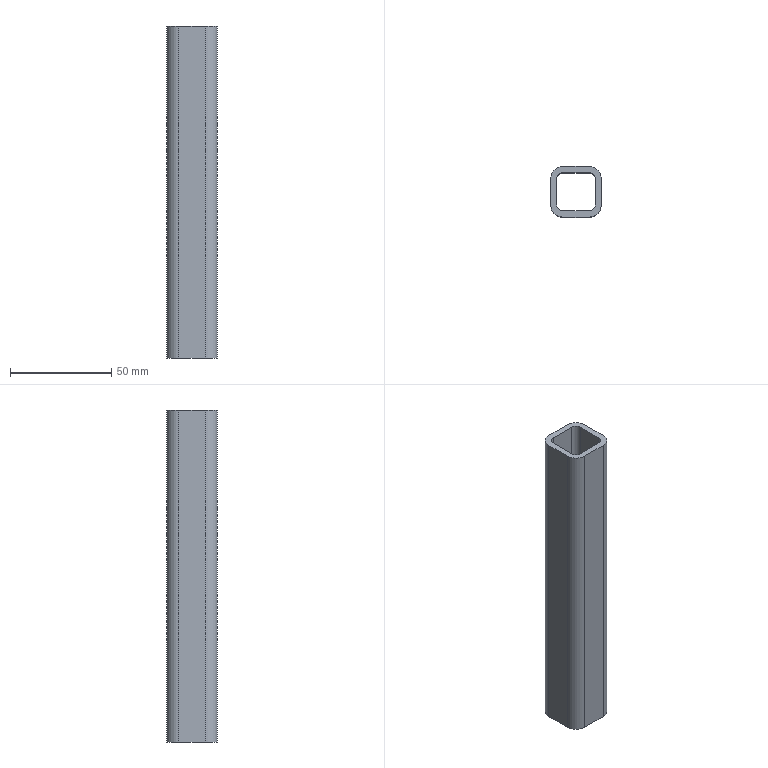Part | STEP file | ISO 10799-2 25x25x3 1784908144036 | 1 solid | 18 faces | box 25 x 25 x 164.089 mm | volume 39516 mm3 | plane 10 | cylinder 8 | commonest cylinder face diameters 6 x4 12 x4
STEP:
#1=CARTESIAN_POINT('',(-6.5,-9.5,164.089));
#2=VERTEX_POINT('',#1);
#3=CARTESIAN_POINT('',(6.5,-9.5,164.089));
#4=VERTEX_POINT('',#3);
#5=CARTESIAN_POINT('',(3.25,-9.5,164.089));
#6=DIRECTION('',(1.,0.,0.));
#7=VECTOR('',#6,10.);
#8=LINE('',#5,#7);
#9=EDGE_CURVE('',#2,#4,#8,.T.);
#10=ORIENTED_EDGE('',*,*,#9,.T.);
#11=CARTESIAN_POINT('',(6.5,-9.5,0.));
#12=VERTEX_POINT('',#11);
#13=CARTESIAN_POINT('',(6.5,-9.5,0.));
#14=DIRECTION('',(0.,0.,1.));
#15=VECTOR('',#14,10.);
#16=LINE('',#13,#15);
#17=EDGE_CURVE('',#12,#4,#16,.T.);
#18=ORIENTED_EDGE('',*,*,#17,.F.);
#19=CARTESIAN_POINT('',(-6.5,-9.5,0.));
#20=VERTEX_POINT('',#19);
#21=CARTESIAN_POINT('',(3.25,-9.5,0.));
#22=DIRECTION('',(1.,0.,0.));
#23=VECTOR('',#22,10.);
#24=LINE('',#21,#23);
#25=EDGE_CURVE('',#20,#12,#24,.T.);
#26=ORIENTED_EDGE('',*,*,#25,.F.);
#27=CARTESIAN_POINT('',(-6.5,-9.5,0.));
#28=DIRECTION('',(0.,0.,1.));
#29=VECTOR('',#28,10.);
#30=LINE('',#27,#29);
#31=EDGE_CURVE('',#20,#2,#30,.T.);
#32=ORIENTED_EDGE('',*,*,#31,.T.);
#33=EDGE_LOOP('',(#10,#18,#26,#32));
#34=FACE_OUTER_BOUND('',#33,.T.);
#35=CARTESIAN_POINT('',(6.5,-9.5,0.));
#36=DIRECTION('',(0.,-1.,0.));
#37=DIRECTION('',(0.,0.,-1.));
#38=AXIS2_PLACEMENT_3D('',#35,#36,#37);
#39=PLANE('',#38);
#40=ADVANCED_FACE('',(#34),#39,.F.);
#41=CARTESIAN_POINT('',(9.5,-6.5,164.089));
#42=VERTEX_POINT('',#41);
#43=CARTESIAN_POINT('',(6.5,-6.5,164.089));
#44=DIRECTION('',(0.,0.,1.));
#45=DIRECTION('',(0.,1.,0.));
#46=AXIS2_PLACEMENT_3D('',#43,#44,#45);
#47=CIRCLE('',#46,3.);
#48=EDGE_CURVE('',#4,#42,#47,.T.);
#49=ORIENTED_EDGE('',*,*,#48,.T.);
#50=CARTESIAN_POINT('',(9.5,-6.5,0.));
#51=VERTEX_POINT('',#50);
#52=CARTESIAN_POINT('',(9.5,-6.5,0.));
#53=DIRECTION('',(0.,0.,1.));
#54=VECTOR('',#53,10.);
#55=LINE('',#52,#54);
#56=EDGE_CURVE('',#51,#42,#55,.T.);
#57=ORIENTED_EDGE('',*,*,#56,.F.);
#58=CARTESIAN_POINT('',(6.5,-6.5,0.));
#59=DIRECTION('',(0.,0.,1.));
#60=DIRECTION('',(0.,1.,0.));
#61=AXIS2_PLACEMENT_3D('',#58,#59,#60);
#62=CIRCLE('',#61,3.);
#63=EDGE_CURVE('',#12,#51,#62,.T.);
#64=ORIENTED_EDGE('',*,*,#63,.F.);
#65=ORIENTED_EDGE('',*,*,#17,.T.);
#66=EDGE_LOOP('',(#49,#57,#64,#65));
#67=FACE_OUTER_BOUND('',#66,.T.);
#68=CARTESIAN_POINT('',(6.5,-6.5,0.));
#69=DIRECTION('',(0.,0.,1.));
#70=DIRECTION('',(0.,1.,0.));
#71=AXIS2_PLACEMENT_3D('',#68,#69,#70);
#72=CYLINDRICAL_SURFACE('',#71,3.);
#73=ADVANCED_FACE('',(#67),#72,.F.);
#74=CARTESIAN_POINT('',(9.5,6.5,164.089));
#75=VERTEX_POINT('',#74);
#76=CARTESIAN_POINT('',(9.5,3.25,164.089));
#77=DIRECTION('',(0.,1.,0.));
#78=VECTOR('',#77,10.);
#79=LINE('',#76,#78);
#80=EDGE_CURVE('',#42,#75,#79,.T.);
#81=ORIENTED_EDGE('',*,*,#80,.T.);
#82=CARTESIAN_POINT('',(9.5,6.5,0.));
#83=VERTEX_POINT('',#82);
#84=CARTESIAN_POINT('',(9.5,6.5,0.));
#85=DIRECTION('',(0.,0.,1.));
#86=VECTOR('',#85,10.);
#87=LINE('',#84,#86);
#88=EDGE_CURVE('',#83,#75,#87,.T.);
#89=ORIENTED_EDGE('',*,*,#88,.F.);
#90=CARTESIAN_POINT('',(9.5,3.25,0.));
#91=DIRECTION('',(0.,1.,0.));
#92=VECTOR('',#91,10.);
#93=LINE('',#90,#92);
#94=EDGE_CURVE('',#51,#83,#93,.T.);
#95=ORIENTED_EDGE('',*,*,#94,.F.);
#96=ORIENTED_EDGE('',*,*,#56,.T.);
#97=EDGE_LOOP('',(#81,#89,#95,#96));
#98=FACE_OUTER_BOUND('',#97,.T.);
#99=CARTESIAN_POINT('',(9.5,6.5,0.));
#100=DIRECTION('',(1.,0.,0.));
#101=DIRECTION('',(0.,0.,-1.));
#102=AXIS2_PLACEMENT_3D('',#99,#100,#101);
#103=PLANE('',#102);
#104=ADVANCED_FACE('',(#98),#103,.F.);
#105=CARTESIAN_POINT('',(6.5,9.5,164.089));
#106=VERTEX_POINT('',#105);
#107=CARTESIAN_POINT('',(6.5,6.5,164.089));
#108=DIRECTION('',(0.,0.,1.));
#109=DIRECTION('',(-1.,0.,0.));
#110=AXIS2_PLACEMENT_3D('',#107,#108,#109);
#111=CIRCLE('',#110,3.);
#112=EDGE_CURVE('',#75,#106,#111,.T.);
#113=ORIENTED_EDGE('',*,*,#112,.T.);
#114=CARTESIAN_POINT('',(6.5,9.5,0.));
#115=VERTEX_POINT('',#114);
#116=CARTESIAN_POINT('',(6.5,9.5,0.));
#117=DIRECTION('',(0.,0.,1.));
#118=VECTOR('',#117,10.);
#119=LINE('',#116,#118);
#120=EDGE_CURVE('',#115,#106,#119,.T.);
#121=ORIENTED_EDGE('',*,*,#120,.F.);
#122=CARTESIAN_POINT('',(6.5,6.5,0.));
#123=DIRECTION('',(0.,0.,1.));
#124=DIRECTION('',(-1.,0.,0.));
#125=AXIS2_PLACEMENT_3D('',#122,#123,#124);
#126=CIRCLE('',#125,3.);
#127=EDGE_CURVE('',#83,#115,#126,.T.);
#128=ORIENTED_EDGE('',*,*,#127,.F.);
#129=ORIENTED_EDGE('',*,*,#88,.T.);
#130=EDGE_LOOP('',(#113,#121,#128,#129));
#131=FACE_OUTER_BOUND('',#130,.T.);
#132=CARTESIAN_POINT('',(6.5,6.5,0.));
#133=DIRECTION('',(0.,0.,1.));
#134=DIRECTION('',(-1.,0.,0.));
#135=AXIS2_PLACEMENT_3D('',#132,#133,#134);
#136=CYLINDRICAL_SURFACE('',#135,3.);
#137=ADVANCED_FACE('',(#131),#136,.F.);
#138=CARTESIAN_POINT('',(12.5,6.5,164.089));
#139=VERTEX_POINT('',#138);
#140=CARTESIAN_POINT('',(12.5,-6.5,164.089));
#141=VERTEX_POINT('',#140);
#142=CARTESIAN_POINT('',(12.5,3.25,164.089));
#143=DIRECTION('',(0.,-1.,0.));
#144=VECTOR('',#143,10.);
#145=LINE('',#142,#144);
#146=EDGE_CURVE('',#139,#141,#145,.T.);
#147=ORIENTED_EDGE('',*,*,#146,.T.);
#148=CARTESIAN_POINT('',(12.5,-6.5,0.));
#149=VERTEX_POINT('',#148);
#150=CARTESIAN_POINT('',(12.5,-6.5,0.));
#151=DIRECTION('',(0.,0.,1.));
#152=VECTOR('',#151,10.);
#153=LINE('',#150,#152);
#154=EDGE_CURVE('',#149,#141,#153,.T.);
#155=ORIENTED_EDGE('',*,*,#154,.F.);
#156=CARTESIAN_POINT('',(12.5,6.5,0.));
#157=VERTEX_POINT('',#156);
#158=CARTESIAN_POINT('',(12.5,3.25,0.));
#159=DIRECTION('',(0.,-1.,0.));
#160=VECTOR('',#159,10.);
#161=LINE('',#158,#160);
#162=EDGE_CURVE('',#157,#149,#161,.T.);
#163=ORIENTED_EDGE('',*,*,#162,.F.);
#164=CARTESIAN_POINT('',(12.5,6.5,0.));
#165=DIRECTION('',(0.,0.,1.));
#166=VECTOR('',#165,10.);
#167=LINE('',#164,#166);
#168=EDGE_CURVE('',#157,#139,#167,.T.);
#169=ORIENTED_EDGE('',*,*,#168,.T.);
#170=EDGE_LOOP('',(#147,#155,#163,#169));
#171=FACE_OUTER_BOUND('',#170,.T.);
#172=CARTESIAN_POINT('',(12.5,6.5,0.));
#173=DIRECTION('',(1.,0.,0.));
#174=DIRECTION('',(0.,0.,-1.));
#175=AXIS2_PLACEMENT_3D('',#172,#173,#174);
#176=PLANE('',#175);
#177=ADVANCED_FACE('',(#171),#176,.T.);
#178=CARTESIAN_POINT('',(6.5,-12.5,164.089));
#179=VERTEX_POINT('',#178);
#180=CARTESIAN_POINT('',(6.5,-6.5,164.089));
#181=DIRECTION('',(0.,0.,-1.));
#182=DIRECTION('',(0.,1.,0.));
#183=AXIS2_PLACEMENT_3D('',#180,#181,#182);
#184=CIRCLE('',#183,6.);
#185=EDGE_CURVE('',#141,#179,#184,.T.);
#186=ORIENTED_EDGE('',*,*,#185,.T.);
#187=CARTESIAN_POINT('',(6.5,-12.5,0.));
#188=VERTEX_POINT('',#187);
#189=CARTESIAN_POINT('',(6.5,-12.5,0.));
#190=DIRECTION('',(0.,0.,1.));
#191=VECTOR('',#190,10.);
#192=LINE('',#189,#191);
#193=EDGE_CURVE('',#188,#179,#192,.T.);
#194=ORIENTED_EDGE('',*,*,#193,.F.);
#195=CARTESIAN_POINT('',(6.5,-6.5,0.));
#196=DIRECTION('',(0.,0.,-1.));
#197=DIRECTION('',(0.,1.,0.));
#198=AXIS2_PLACEMENT_3D('',#195,#196,#197);
#199=CIRCLE('',#198,6.);
#200=EDGE_CURVE('',#149,#188,#199,.T.);
#201=ORIENTED_EDGE('',*,*,#200,.F.);
#202=ORIENTED_EDGE('',*,*,#154,.T.);
#203=EDGE_LOOP('',(#186,#194,#201,#202));
#204=FACE_OUTER_BOUND('',#203,.T.);
#205=CARTESIAN_POINT('',(6.5,-6.5,0.));
#206=DIRECTION('',(0.,0.,1.));
#207=DIRECTION('',(0.,1.,0.));
#208=AXIS2_PLACEMENT_3D('',#205,#206,#207);
#209=CYLINDRICAL_SURFACE('',#208,6.);
#210=ADVANCED_FACE('',(#204),#209,.T.);
#211=CARTESIAN_POINT('',(-6.5,-12.5,164.089));
#212=VERTEX_POINT('',#211);
#213=CARTESIAN_POINT('',(3.25,-12.5,164.089));
#214=DIRECTION('',(-1.,0.,0.));
#215=VECTOR('',#214,10.);
#216=LINE('',#213,#215);
#217=EDGE_CURVE('',#179,#212,#216,.T.);
#218=ORIENTED_EDGE('',*,*,#217,.T.);
#219=CARTESIAN_POINT('',(-6.5,-12.5,0.));
#220=VERTEX_POINT('',#219);
#221=CARTESIAN_POINT('',(-6.5,-12.5,0.));
#222=DIRECTION('',(0.,0.,1.));
#223=VECTOR('',#222,10.);
#224=LINE('',#221,#223);
#225=EDGE_CURVE('',#220,#212,#224,.T.);
#226=ORIENTED_EDGE('',*,*,#225,.F.);
#227=CARTESIAN_POINT('',(3.25,-12.5,0.));
#228=DIRECTION('',(-1.,0.,0.));
#229=VECTOR('',#228,10.);
#230=LINE('',#227,#229);
#231=EDGE_CURVE('',#188,#220,#230,.T.);
#232=ORIENTED_EDGE('',*,*,#231,.F.);
#233=ORIENTED_EDGE('',*,*,#193,.T.);
#234=EDGE_LOOP('',(#218,#226,#232,#233));
#235=FACE_OUTER_BOUND('',#234,.T.);
#236=CARTESIAN_POINT('',(6.5,-12.5,0.));
#237=DIRECTION('',(0.,-1.,0.));
#238=DIRECTION('',(0.,0.,-1.));
#239=AXIS2_PLACEMENT_3D('',#236,#237,#238);
#240=PLANE('',#239);
#241=ADVANCED_FACE('',(#235),#240,.T.);
#242=CARTESIAN_POINT('',(-12.5,-6.5,164.089));
#243=VERTEX_POINT('',#242);
#244=CARTESIAN_POINT('',(-6.5,-6.5,164.089));
#245=DIRECTION('',(0.,0.,-1.));
#246=DIRECTION('',(1.,0.,0.));
#247=AXIS2_PLACEMENT_3D('',#244,#245,#246);
#248=CIRCLE('',#247,6.);
#249=EDGE_CURVE('',#212,#243,#248,.T.);
#250=ORIENTED_EDGE('',*,*,#249,.T.);
#251=CARTESIAN_POINT('',(-12.5,-6.5,0.));
#252=VERTEX_POINT('',#251);
#253=CARTESIAN_POINT('',(-12.5,-6.5,0.));
#254=DIRECTION('',(0.,0.,1.));
#255=VECTOR('',#254,10.);
#256=LINE('',#253,#255);
#257=EDGE_CURVE('',#252,#243,#256,.T.);
#258=ORIENTED_EDGE('',*,*,#257,.F.);
#259=CARTESIAN_POINT('',(-6.5,-6.5,0.));
#260=DIRECTION('',(0.,0.,-1.));
#261=DIRECTION('',(1.,0.,0.));
#262=AXIS2_PLACEMENT_3D('',#259,#260,#261);
#263=CIRCLE('',#262,6.);
#264=EDGE_CURVE('',#220,#252,#263,.T.);
#265=ORIENTED_EDGE('',*,*,#264,.F.);
#266=ORIENTED_EDGE('',*,*,#225,.T.);
#267=EDGE_LOOP('',(#250,#258,#265,#266));
#268=FACE_OUTER_BOUND('',#267,.T.);
#269=CARTESIAN_POINT('',(-6.5,-6.5,0.));
#270=DIRECTION('',(0.,0.,1.));
#271=DIRECTION('',(1.,0.,0.));
#272=AXIS2_PLACEMENT_3D('',#269,#270,#271);
#273=CYLINDRICAL_SURFACE('',#272,6.);
#274=ADVANCED_FACE('',(#268),#273,.T.);
#275=CARTESIAN_POINT('',(-6.5,9.5,164.089));
#276=VERTEX_POINT('',#275);
#277=CARTESIAN_POINT('',(-3.25,9.5,164.089));
#278=DIRECTION('',(-1.,0.,0.));
#279=VECTOR('',#278,10.);
#280=LINE('',#277,#279);
#281=EDGE_CURVE('',#106,#276,#280,.T.);
#282=ORIENTED_EDGE('',*,*,#281,.T.);
#283=CARTESIAN_POINT('',(-6.5,9.5,0.));
#284=VERTEX_POINT('',#283);
#285=CARTESIAN_POINT('',(-6.5,9.5,0.));
#286=DIRECTION('',(0.,0.,1.));
#287=VECTOR('',#286,10.);
#288=LINE('',#285,#287);
#289=EDGE_CURVE('',#284,#276,#288,.T.);
#290=ORIENTED_EDGE('',*,*,#289,.F.);
#291=CARTESIAN_POINT('',(-3.25,9.5,0.));
#292=DIRECTION('',(-1.,0.,0.));
#293=VECTOR('',#292,10.);
#294=LINE('',#291,#293);
#295=EDGE_CURVE('',#115,#284,#294,.T.);
#296=ORIENTED_EDGE('',*,*,#295,.F.);
#297=ORIENTED_EDGE('',*,*,#120,.T.);
#298=EDGE_LOOP('',(#282,#290,#296,#297));
#299=FACE_OUTER_BOUND('',#298,.T.);
#300=CARTESIAN_POINT('',(-6.5,9.5,0.));
#301=DIRECTION('',(0.,1.,0.));
#302=DIRECTION('',(0.,0.,1.));
#303=AXIS2_PLACEMENT_3D('',#300,#301,#302);
#304=PLANE('',#303);
#305=ADVANCED_FACE('',(#299),#304,.F.);
#306=CARTESIAN_POINT('',(-9.5,-6.5,164.089));
#307=VERTEX_POINT('',#306);
#308=CARTESIAN_POINT('',(-6.5,-6.5,164.089));
#309=DIRECTION('',(0.,0.,1.));
#310=DIRECTION('',(1.,0.,0.));
#311=AXIS2_PLACEMENT_3D('',#308,#309,#310);
#312=CIRCLE('',#311,3.);
#313=EDGE_CURVE('',#307,#2,#312,.T.);
#314=ORIENTED_EDGE('',*,*,#313,.T.);
#315=ORIENTED_EDGE('',*,*,#31,.F.);
#316=CARTESIAN_POINT('',(-9.5,-6.5,0.));
#317=VERTEX_POINT('',#316);
#318=CARTESIAN_POINT('',(-6.5,-6.5,0.));
#319=DIRECTION('',(0.,0.,1.));
#320=DIRECTION('',(1.,0.,0.));
#321=AXIS2_PLACEMENT_3D('',#318,#319,#320);
#322=CIRCLE('',#321,3.);
#323=EDGE_CURVE('',#317,#20,#322,.T.);
#324=ORIENTED_EDGE('',*,*,#323,.F.);
#325=CARTESIAN_POINT('',(-9.5,-6.5,0.));
#326=DIRECTION('',(0.,0.,1.));
#327=VECTOR('',#326,10.);
#328=LINE('',#325,#327);
#329=EDGE_CURVE('',#317,#307,#328,.T.);
#330=ORIENTED_EDGE('',*,*,#329,.T.);
#331=EDGE_LOOP('',(#314,#315,#324,#330));
#332=FACE_OUTER_BOUND('',#331,.T.);
#333=CARTESIAN_POINT('',(-6.5,-6.5,0.));
#334=DIRECTION('',(0.,0.,1.));
#335=DIRECTION('',(1.,0.,0.));
#336=AXIS2_PLACEMENT_3D('',#333,#334,#335);
#337=CYLINDRICAL_SURFACE('',#336,3.);
#338=ADVANCED_FACE('',(#332),#337,.F.);
#339=CARTESIAN_POINT('',(-9.5,6.5,164.089));
#340=VERTEX_POINT('',#339);
#341=CARTESIAN_POINT('',(-9.5,-3.25,164.089));
#342=DIRECTION('',(0.,-1.,0.));
#343=VECTOR('',#342,10.);
#344=LINE('',#341,#343);
#345=EDGE_CURVE('',#340,#307,#344,.T.);
#346=ORIENTED_EDGE('',*,*,#345,.T.);
#347=ORIENTED_EDGE('',*,*,#329,.F.);
#348=CARTESIAN_POINT('',(-9.5,6.5,0.));
#349=VERTEX_POINT('',#348);
#350=CARTESIAN_POINT('',(-9.5,-3.25,0.));
#351=DIRECTION('',(0.,-1.,0.));
#352=VECTOR('',#351,10.);
#353=LINE('',#350,#352);
#354=EDGE_CURVE('',#349,#317,#353,.T.);
#355=ORIENTED_EDGE('',*,*,#354,.F.);
#356=CARTESIAN_POINT('',(-9.5,6.5,0.));
#357=DIRECTION('',(0.,0.,1.));
#358=VECTOR('',#357,10.);
#359=LINE('',#356,#358);
#360=EDGE_CURVE('',#349,#340,#359,.T.);
#361=ORIENTED_EDGE('',*,*,#360,.T.);
#362=EDGE_LOOP('',(#346,#347,#355,#361));
#363=FACE_OUTER_BOUND('',#362,.T.);
#364=CARTESIAN_POINT('',(-9.5,-6.5,0.));
#365=DIRECTION('',(-1.,0.,0.));
#366=DIRECTION('',(0.,0.,1.));
#367=AXIS2_PLACEMENT_3D('',#364,#365,#366);
#368=PLANE('',#367);
#369=ADVANCED_FACE('',(#363),#368,.F.);
#370=CARTESIAN_POINT('',(-6.5,6.5,164.089));
#371=DIRECTION('',(0.,0.,1.));
#372=DIRECTION('',(0.,-1.,0.));
#373=AXIS2_PLACEMENT_3D('',#370,#371,#372);
#374=CIRCLE('',#373,3.);
#375=EDGE_CURVE('',#276,#340,#374,.T.);
#376=ORIENTED_EDGE('',*,*,#375,.T.);
#377=ORIENTED_EDGE('',*,*,#360,.F.);
#378=CARTESIAN_POINT('',(-6.5,6.5,0.));
#379=DIRECTION('',(0.,0.,1.));
#380=DIRECTION('',(0.,-1.,0.));
#381=AXIS2_PLACEMENT_3D('',#378,#379,#380);
#382=CIRCLE('',#381,3.);
#383=EDGE_CURVE('',#284,#349,#382,.T.);
#384=ORIENTED_EDGE('',*,*,#383,.F.);
#385=ORIENTED_EDGE('',*,*,#289,.T.);
#386=EDGE_LOOP('',(#376,#377,#384,#385));
#387=FACE_OUTER_BOUND('',#386,.T.);
#388=CARTESIAN_POINT('',(-6.5,6.5,0.));
#389=DIRECTION('',(0.,0.,1.));
#390=DIRECTION('',(0.,-1.,0.));
#391=AXIS2_PLACEMENT_3D('',#388,#389,#390);
#392=CYLINDRICAL_SURFACE('',#391,3.);
#393=ADVANCED_FACE('',(#387),#392,.F.);
#394=CARTESIAN_POINT('',(-12.5,6.5,164.089));
#395=VERTEX_POINT('',#394);
#396=CARTESIAN_POINT('',(-12.5,-3.25,164.089));
#397=DIRECTION('',(0.,1.,0.));
#398=VECTOR('',#397,10.);
#399=LINE('',#396,#398);
#400=EDGE_CURVE('',#243,#395,#399,.T.);
#401=ORIENTED_EDGE('',*,*,#400,.T.);
#402=CARTESIAN_POINT('',(-12.5,6.5,0.));
#403=VERTEX_POINT('',#402);
#404=CARTESIAN_POINT('',(-12.5,6.5,0.));
#405=DIRECTION('',(0.,0.,1.));
#406=VECTOR('',#405,10.);
#407=LINE('',#404,#406);
#408=EDGE_CURVE('',#403,#395,#407,.T.);
#409=ORIENTED_EDGE('',*,*,#408,.F.);
#410=CARTESIAN_POINT('',(-12.5,-3.25,0.));
#411=DIRECTION('',(0.,1.,0.));
#412=VECTOR('',#411,10.);
#413=LINE('',#410,#412);
#414=EDGE_CURVE('',#252,#403,#413,.T.);
#415=ORIENTED_EDGE('',*,*,#414,.F.);
#416=ORIENTED_EDGE('',*,*,#257,.T.);
#417=EDGE_LOOP('',(#401,#409,#415,#416));
#418=FACE_OUTER_BOUND('',#417,.T.);
#419=CARTESIAN_POINT('',(-12.5,-6.5,0.));
#420=DIRECTION('',(-1.,0.,0.));
#421=DIRECTION('',(0.,0.,1.));
#422=AXIS2_PLACEMENT_3D('',#419,#420,#421);
#423=PLANE('',#422);
#424=ADVANCED_FACE('',(#418),#423,.T.);
#425=CARTESIAN_POINT('',(-6.5,12.5,164.089));
#426=VERTEX_POINT('',#425);
#427=CARTESIAN_POINT('',(-6.5,6.5,164.089));
#428=DIRECTION('',(0.,0.,-1.));
#429=DIRECTION('',(0.,-1.,0.));
#430=AXIS2_PLACEMENT_3D('',#427,#428,#429);
#431=CIRCLE('',#430,6.);
#432=EDGE_CURVE('',#395,#426,#431,.T.);
#433=ORIENTED_EDGE('',*,*,#432,.T.);
#434=CARTESIAN_POINT('',(-6.5,12.5,0.));
#435=VERTEX_POINT('',#434);
#436=CARTESIAN_POINT('',(-6.5,12.5,0.));
#437=DIRECTION('',(0.,0.,1.));
#438=VECTOR('',#437,10.);
#439=LINE('',#436,#438);
#440=EDGE_CURVE('',#435,#426,#439,.T.);
#441=ORIENTED_EDGE('',*,*,#440,.F.);
#442=CARTESIAN_POINT('',(-6.5,6.5,0.));
#443=DIRECTION('',(0.,0.,-1.));
#444=DIRECTION('',(0.,-1.,0.));
#445=AXIS2_PLACEMENT_3D('',#442,#443,#444);
#446=CIRCLE('',#445,6.);
#447=EDGE_CURVE('',#403,#435,#446,.T.);
#448=ORIENTED_EDGE('',*,*,#447,.F.);
#449=ORIENTED_EDGE('',*,*,#408,.T.);
#450=EDGE_LOOP('',(#433,#441,#448,#449));
#451=FACE_OUTER_BOUND('',#450,.T.);
#452=CARTESIAN_POINT('',(-6.5,6.5,0.));
#453=DIRECTION('',(0.,0.,1.));
#454=DIRECTION('',(0.,-1.,0.));
#455=AXIS2_PLACEMENT_3D('',#452,#453,#454);
#456=CYLINDRICAL_SURFACE('',#455,6.);
#457=ADVANCED_FACE('',(#451),#456,.T.);
#458=CARTESIAN_POINT('',(6.5,12.5,164.089));
#459=VERTEX_POINT('',#458);
#460=CARTESIAN_POINT('',(-3.25,12.5,164.089));
#461=DIRECTION('',(1.,0.,0.));
#462=VECTOR('',#461,10.);
#463=LINE('',#460,#462);
#464=EDGE_CURVE('',#426,#459,#463,.T.);
#465=ORIENTED_EDGE('',*,*,#464,.T.);
#466=CARTESIAN_POINT('',(6.5,12.5,0.));
#467=VERTEX_POINT('',#466);
#468=CARTESIAN_POINT('',(6.5,12.5,0.));
#469=DIRECTION('',(0.,0.,1.));
#470=VECTOR('',#469,10.);
#471=LINE('',#468,#470);
#472=EDGE_CURVE('',#467,#459,#471,.T.);
#473=ORIENTED_EDGE('',*,*,#472,.F.);
#474=CARTESIAN_POINT('',(-3.25,12.5,0.));
#475=DIRECTION('',(1.,0.,0.));
#476=VECTOR('',#475,10.);
#477=LINE('',#474,#476);
#478=EDGE_CURVE('',#435,#467,#477,.T.);
#479=ORIENTED_EDGE('',*,*,#478,.F.);
#480=ORIENTED_EDGE('',*,*,#440,.T.);
#481=EDGE_LOOP('',(#465,#473,#479,#480));
#482=FACE_OUTER_BOUND('',#481,.T.);
#483=CARTESIAN_POINT('',(-6.5,12.5,0.));
#484=DIRECTION('',(0.,1.,0.));
#485=DIRECTION('',(0.,0.,1.));
#486=AXIS2_PLACEMENT_3D('',#483,#484,#485);
#487=PLANE('',#486);
#488=ADVANCED_FACE('',(#482),#487,.T.);
#489=CARTESIAN_POINT('',(6.5,6.5,164.089));
#490=DIRECTION('',(0.,0.,-1.));
#491=DIRECTION('',(-1.,0.,0.));
#492=AXIS2_PLACEMENT_3D('',#489,#490,#491);
#493=CIRCLE('',#492,6.);
#494=EDGE_CURVE('',#459,#139,#493,.T.);
#495=ORIENTED_EDGE('',*,*,#494,.T.);
#496=ORIENTED_EDGE('',*,*,#168,.F.);
#497=CARTESIAN_POINT('',(6.5,6.5,0.));
#498=DIRECTION('',(0.,0.,-1.));
#499=DIRECTION('',(-1.,0.,0.));
#500=AXIS2_PLACEMENT_3D('',#497,#498,#499);
#501=CIRCLE('',#500,6.);
#502=EDGE_CURVE('',#467,#157,#501,.T.);
#503=ORIENTED_EDGE('',*,*,#502,.F.);
#504=ORIENTED_EDGE('',*,*,#472,.T.);
#505=EDGE_LOOP('',(#495,#496,#503,#504));
#506=FACE_OUTER_BOUND('',#505,.T.);
#507=CARTESIAN_POINT('',(6.5,6.5,0.));
#508=DIRECTION('',(0.,0.,1.));
#509=DIRECTION('',(-1.,0.,0.));
#510=AXIS2_PLACEMENT_3D('',#507,#508,#509);
#511=CYLINDRICAL_SURFACE('',#510,6.);
#512=ADVANCED_FACE('',(#506),#511,.T.);
#513=ORIENTED_EDGE('',*,*,#414,.T.);
#514=ORIENTED_EDGE('',*,*,#447,.T.);
#515=ORIENTED_EDGE('',*,*,#478,.T.);
#516=ORIENTED_EDGE('',*,*,#502,.T.);
#517=ORIENTED_EDGE('',*,*,#162,.T.);
#518=ORIENTED_EDGE('',*,*,#200,.T.);
#519=ORIENTED_EDGE('',*,*,#231,.T.);
#520=ORIENTED_EDGE('',*,*,#264,.T.);
#521=EDGE_LOOP('',(#513,#514,#515,#516,#517,#518,#519,#520));
#522=FACE_OUTER_BOUND('',#521,.T.);
#523=ORIENTED_EDGE('',*,*,#295,.T.);
#524=ORIENTED_EDGE('',*,*,#383,.T.);
#525=ORIENTED_EDGE('',*,*,#354,.T.);
#526=ORIENTED_EDGE('',*,*,#323,.T.);
#527=ORIENTED_EDGE('',*,*,#25,.T.);
#528=ORIENTED_EDGE('',*,*,#63,.T.);
#529=ORIENTED_EDGE('',*,*,#94,.T.);
#530=ORIENTED_EDGE('',*,*,#127,.T.);
#531=EDGE_LOOP('',(#523,#524,#525,#526,#527,#528,#529,#530));
#532=FACE_BOUND('',#531,.T.);
#533=CARTESIAN_POINT('',(0.,0.,0.));
#534=DIRECTION('',(0.,0.,1.));
#535=DIRECTION('',(1.,0.,0.));
#536=AXIS2_PLACEMENT_3D('',#533,#534,#535);
#537=PLANE('',#536);
#538=ADVANCED_FACE('',(#522,#532),#537,.F.);
#539=ORIENTED_EDGE('',*,*,#400,.F.);
#540=ORIENTED_EDGE('',*,*,#249,.F.);
#541=ORIENTED_EDGE('',*,*,#217,.F.);
#542=ORIENTED_EDGE('',*,*,#185,.F.);
#543=ORIENTED_EDGE('',*,*,#146,.F.);
#544=ORIENTED_EDGE('',*,*,#494,.F.);
#545=ORIENTED_EDGE('',*,*,#464,.F.);
#546=ORIENTED_EDGE('',*,*,#432,.F.);
#547=EDGE_LOOP('',(#539,#540,#541,#542,#543,#544,#545,#546));
#548=FACE_OUTER_BOUND('',#547,.T.);
#549=ORIENTED_EDGE('',*,*,#281,.F.);
#550=ORIENTED_EDGE('',*,*,#112,.F.);
#551=ORIENTED_EDGE('',*,*,#80,.F.);
#552=ORIENTED_EDGE('',*,*,#48,.F.);
#553=ORIENTED_EDGE('',*,*,#9,.F.);
#554=ORIENTED_EDGE('',*,*,#313,.F.);
#555=ORIENTED_EDGE('',*,*,#345,.F.);
#556=ORIENTED_EDGE('',*,*,#375,.F.);
#557=EDGE_LOOP('',(#549,#550,#551,#552,#553,#554,#555,#556));
#558=FACE_BOUND('',#557,.T.);
#559=CARTESIAN_POINT('',(0.,0.,164.089));
#560=DIRECTION('',(0.,0.,1.));
#561=DIRECTION('',(1.,0.,0.));
#562=AXIS2_PLACEMENT_3D('',#559,#560,#561);
#563=PLANE('',#562);
#564=ADVANCED_FACE('',(#548,#558),#563,.T.);
#565=CLOSED_SHELL('',(#40,#73,#104,#137,#177,#210,#241,#274,#305,#338,#369,#393,#424,#457,#488,#512,#538,#564));
#566=MANIFOLD_SOLID_BREP('',#565);
#567=(LENGTH_UNIT()NAMED_UNIT(*)SI_UNIT(.MILLI.,.METRE.));
#568=UNCERTAINTY_MEASURE_WITH_UNIT(LENGTH_MEASURE(0.01),#567,'','');
#569=(NAMED_UNIT(*)PLANE_ANGLE_UNIT()SI_UNIT($,.RADIAN.));
#570=(NAMED_UNIT(*)SI_UNIT($,.STERADIAN.)SOLID_ANGLE_UNIT());
#571=(GEOMETRIC_REPRESENTATION_CONTEXT(3)GLOBAL_UNCERTAINTY_ASSIGNED_CONTEXT((#568))GLOBAL_UNIT_ASSIGNED_CONTEXT((#567,#569,#570))REPRESENTATION_CONTEXT('',''));
#572=ADVANCED_BREP_SHAPE_REPRESENTATION('',(#566),#571);